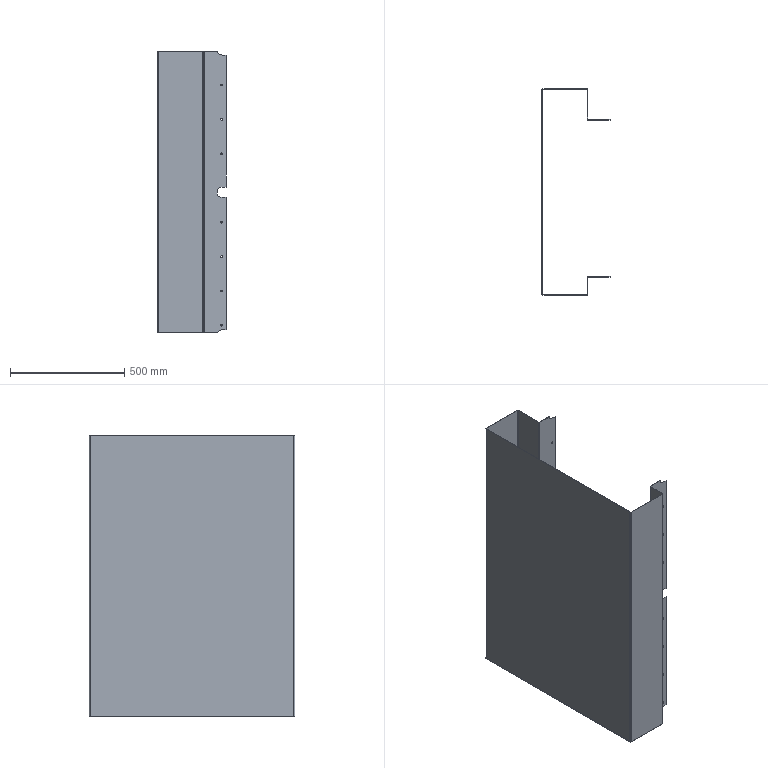Part | STEP file | C3 | 1 solid | 60 faces | box 298.717 x 900 x 1230 mm | volume 3124708 mm3 | cylinder 32 | plane 28 | commonest cylinder face diameters 7 x18 45 x6 4 x4 6 x2 10 x2